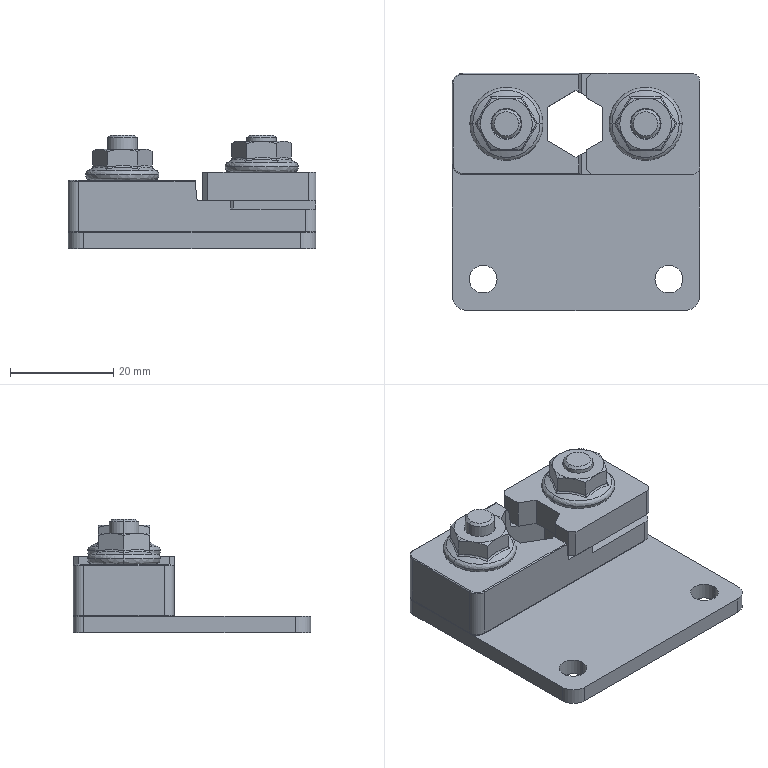Part | SolidWorks | features BaseBody 7 | 7 solids | 273 faces | box 48 x 46 x 22 mm | volume 16357 mm3 | cone 110 | cylinder 70 | plane 67 | spline 26 | commonest cylinder face diameters 4.917 x32 5.7 x8 0.4 x7 4 x6 5.38 x4 6.2 x4